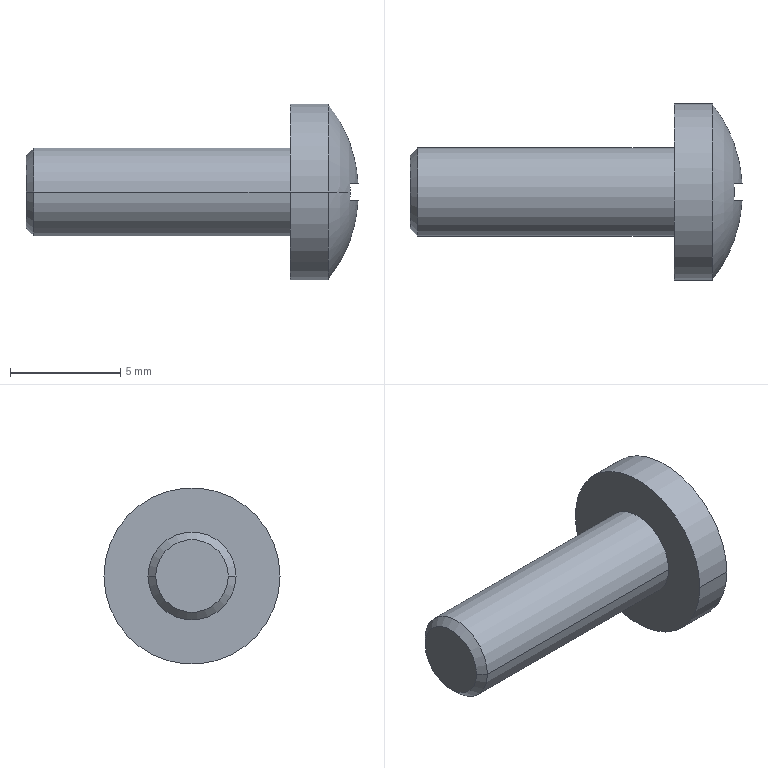Part | STEP file | SOLID | 1 solid | 23 faces | box 15.088 x 8 x 8 mm | volume 268.486 mm3 | plane 15 | cylinder 4 | sphere 2 | cone 2 | commonest cylinder face diameters 4 x2 8 x2